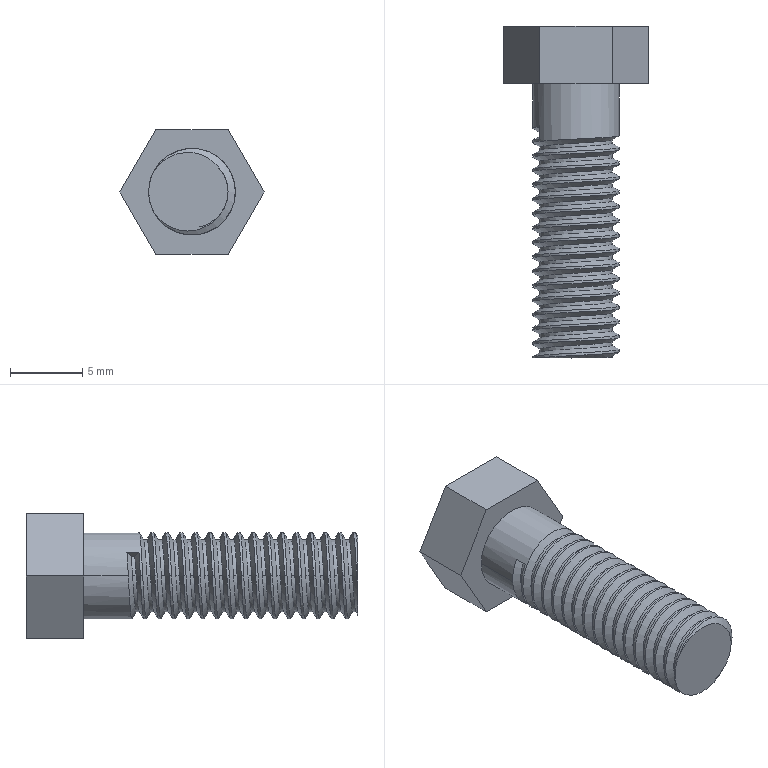Part | SolidWorks | features BaseBody 1 | 1 solid | 78 faces | box 10 x 23 x 8.66 mm | volume 722.509 mm3 | cylinder 66 | plane 10 | spline 2 | commonest cylinder face diameters 5 x33 6 x33